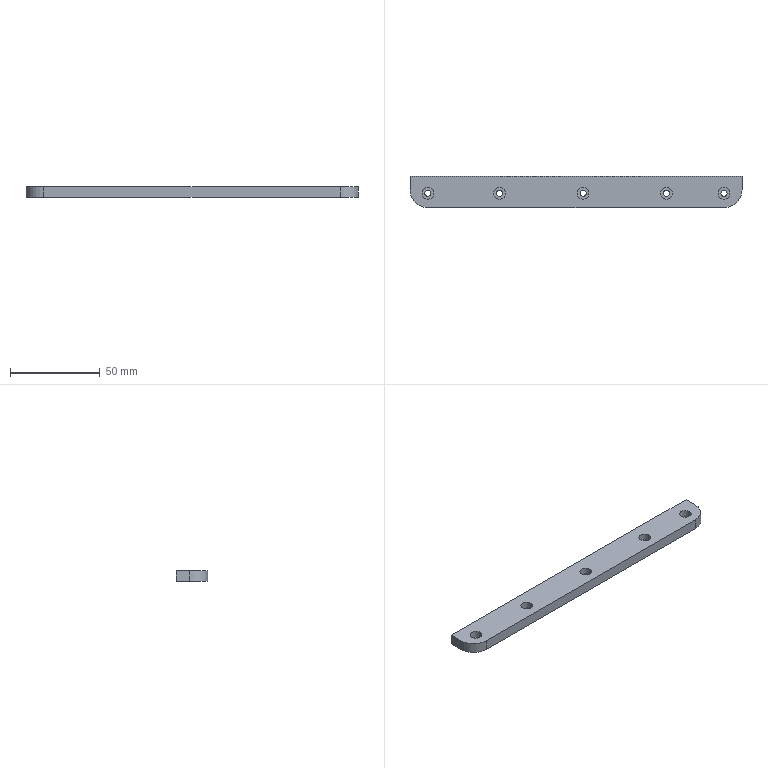Part | STEP file | 229H151433 Default | 1 solid | 33 faces | box 185 x 17.5 x 6 mm | volume 18413 mm3 | cylinder 22 | plane 11 | commonest cylinder face diameters 3.4 x10 6.5 x10 20 x2
STEP:
#1=CARTESIAN_POINT('',(79.209,-0.75,2.));
#2=VERTEX_POINT('',#1);
#3=CARTESIAN_POINT('',(85.709,-0.75,2.));
#4=VERTEX_POINT('',#3);
#5=CARTESIAN_POINT('',(82.459,-0.75,2.));
#6=DIRECTION('',(0.,0.,1.));
#7=DIRECTION('',(1.,0.,0.));
#8=AXIS2_PLACEMENT_3D('',#5,#6,#7);
#9=CIRCLE('',#8,3.25);
#10=EDGE_CURVE('',#2,#4,#9,.T.);
#11=ORIENTED_EDGE('',*,*,#10,.F.);
#12=CARTESIAN_POINT('',(79.209,-0.75,6.));
#13=VERTEX_POINT('',#12);
#14=CARTESIAN_POINT('',(79.209,-0.75,6.));
#15=DIRECTION('',(0.,0.,1.));
#16=VECTOR('',#15,1000.);
#17=LINE('',#14,#16);
#18=EDGE_CURVE('',#2,#13,#17,.T.);
#19=ORIENTED_EDGE('',*,*,#18,.T.);
#20=CARTESIAN_POINT('',(85.709,-0.75,6.));
#21=VERTEX_POINT('',#20);
#22=CARTESIAN_POINT('',(82.459,-0.75,6.));
#23=DIRECTION('',(0.,0.,1.));
#24=DIRECTION('',(1.,0.,0.));
#25=AXIS2_PLACEMENT_3D('',#22,#23,#24);
#26=CIRCLE('',#25,3.25);
#27=EDGE_CURVE('',#13,#21,#26,.T.);
#28=ORIENTED_EDGE('',*,*,#27,.T.);
#29=CARTESIAN_POINT('',(85.709,-0.75,6.));
#30=DIRECTION('',(0.,0.,1.));
#31=VECTOR('',#30,1000.);
#32=LINE('',#29,#31);
#33=EDGE_CURVE('',#4,#21,#32,.T.);
#34=ORIENTED_EDGE('',*,*,#33,.F.);
#35=EDGE_LOOP('',(#11,#19,#28,#34));
#36=FACE_OUTER_BOUND('',#35,.T.);
#37=CARTESIAN_POINT('',(82.459,-0.75,6.));
#38=DIRECTION('',(0.,0.,1.));
#39=DIRECTION('',(1.,0.,0.));
#40=AXIS2_PLACEMENT_3D('',#37,#38,#39);
#41=CYLINDRICAL_SURFACE('',#40,3.25);
#42=ADVANCED_FACE('',(#36),#41,.F.);
#43=CARTESIAN_POINT('',(80.759,-0.75,0.));
#44=VERTEX_POINT('',#43);
#45=CARTESIAN_POINT('',(84.159,-0.75,0.));
#46=VERTEX_POINT('',#45);
#47=CARTESIAN_POINT('',(82.459,-0.75,0.));
#48=DIRECTION('',(0.,0.,1.));
#49=DIRECTION('',(1.,0.,0.));
#50=AXIS2_PLACEMENT_3D('',#47,#48,#49);
#51=CIRCLE('',#50,1.7);
#52=EDGE_CURVE('',#44,#46,#51,.T.);
#53=ORIENTED_EDGE('',*,*,#52,.F.);
#54=CARTESIAN_POINT('',(80.759,-0.75,2.));
#55=VERTEX_POINT('',#54);
#56=CARTESIAN_POINT('',(80.759,-0.75,6.));
#57=DIRECTION('',(0.,0.,1.));
#58=VECTOR('',#57,1000.);
#59=LINE('',#56,#58);
#60=EDGE_CURVE('',#44,#55,#59,.T.);
#61=ORIENTED_EDGE('',*,*,#60,.T.);
#62=CARTESIAN_POINT('',(84.159,-0.75,2.));
#63=VERTEX_POINT('',#62);
#64=CARTESIAN_POINT('',(82.459,-0.75,2.));
#65=DIRECTION('',(0.,0.,1.));
#66=DIRECTION('',(1.,0.,0.));
#67=AXIS2_PLACEMENT_3D('',#64,#65,#66);
#68=CIRCLE('',#67,1.7);
#69=EDGE_CURVE('',#55,#63,#68,.T.);
#70=ORIENTED_EDGE('',*,*,#69,.T.);
#71=CARTESIAN_POINT('',(84.159,-0.75,6.));
#72=DIRECTION('',(0.,0.,1.));
#73=VECTOR('',#72,1000.);
#74=LINE('',#71,#73);
#75=EDGE_CURVE('',#46,#63,#74,.T.);
#76=ORIENTED_EDGE('',*,*,#75,.F.);
#77=EDGE_LOOP('',(#53,#61,#70,#76));
#78=FACE_OUTER_BOUND('',#77,.T.);
#79=CARTESIAN_POINT('',(82.459,-0.75,6.));
#80=DIRECTION('',(0.,0.,1.));
#81=DIRECTION('',(1.,0.,0.));
#82=AXIS2_PLACEMENT_3D('',#79,#80,#81);
#83=CYLINDRICAL_SURFACE('',#82,1.7);
#84=ADVANCED_FACE('',(#78),#83,.F.);
#85=CARTESIAN_POINT('',(47.209,-0.75,2.));
#86=VERTEX_POINT('',#85);
#87=CARTESIAN_POINT('',(53.709,-0.75,2.));
#88=VERTEX_POINT('',#87);
#89=CARTESIAN_POINT('',(50.459,-0.75,2.));
#90=DIRECTION('',(0.,0.,1.));
#91=DIRECTION('',(1.,0.,0.));
#92=AXIS2_PLACEMENT_3D('',#89,#90,#91);
#93=CIRCLE('',#92,3.25);
#94=EDGE_CURVE('',#86,#88,#93,.T.);
#95=ORIENTED_EDGE('',*,*,#94,.F.);
#96=CARTESIAN_POINT('',(47.209,-0.75,6.));
#97=VERTEX_POINT('',#96);
#98=CARTESIAN_POINT('',(47.209,-0.75,6.));
#99=DIRECTION('',(0.,0.,1.));
#100=VECTOR('',#99,1000.);
#101=LINE('',#98,#100);
#102=EDGE_CURVE('',#86,#97,#101,.T.);
#103=ORIENTED_EDGE('',*,*,#102,.T.);
#104=CARTESIAN_POINT('',(53.709,-0.75,6.));
#105=VERTEX_POINT('',#104);
#106=CARTESIAN_POINT('',(50.459,-0.75,6.));
#107=DIRECTION('',(0.,0.,1.));
#108=DIRECTION('',(1.,0.,0.));
#109=AXIS2_PLACEMENT_3D('',#106,#107,#108);
#110=CIRCLE('',#109,3.25);
#111=EDGE_CURVE('',#97,#105,#110,.T.);
#112=ORIENTED_EDGE('',*,*,#111,.T.);
#113=CARTESIAN_POINT('',(53.709,-0.75,6.));
#114=DIRECTION('',(0.,0.,1.));
#115=VECTOR('',#114,1000.);
#116=LINE('',#113,#115);
#117=EDGE_CURVE('',#88,#105,#116,.T.);
#118=ORIENTED_EDGE('',*,*,#117,.F.);
#119=EDGE_LOOP('',(#95,#103,#112,#118));
#120=FACE_OUTER_BOUND('',#119,.T.);
#121=CARTESIAN_POINT('',(50.459,-0.75,6.));
#122=DIRECTION('',(0.,0.,1.));
#123=DIRECTION('',(1.,0.,0.));
#124=AXIS2_PLACEMENT_3D('',#121,#122,#123);
#125=CYLINDRICAL_SURFACE('',#124,3.25);
#126=ADVANCED_FACE('',(#120),#125,.F.);
#127=CARTESIAN_POINT('',(48.759,-0.75,0.));
#128=VERTEX_POINT('',#127);
#129=CARTESIAN_POINT('',(52.159,-0.75,0.));
#130=VERTEX_POINT('',#129);
#131=CARTESIAN_POINT('',(50.459,-0.75,0.));
#132=DIRECTION('',(0.,0.,1.));
#133=DIRECTION('',(1.,0.,0.));
#134=AXIS2_PLACEMENT_3D('',#131,#132,#133);
#135=CIRCLE('',#134,1.7);
#136=EDGE_CURVE('',#128,#130,#135,.T.);
#137=ORIENTED_EDGE('',*,*,#136,.F.);
#138=CARTESIAN_POINT('',(48.759,-0.75,2.));
#139=VERTEX_POINT('',#138);
#140=CARTESIAN_POINT('',(48.759,-0.75,6.));
#141=DIRECTION('',(0.,0.,1.));
#142=VECTOR('',#141,1000.);
#143=LINE('',#140,#142);
#144=EDGE_CURVE('',#128,#139,#143,.T.);
#145=ORIENTED_EDGE('',*,*,#144,.T.);
#146=CARTESIAN_POINT('',(52.159,-0.75,2.));
#147=VERTEX_POINT('',#146);
#148=CARTESIAN_POINT('',(50.459,-0.75,2.));
#149=DIRECTION('',(0.,0.,1.));
#150=DIRECTION('',(1.,0.,0.));
#151=AXIS2_PLACEMENT_3D('',#148,#149,#150);
#152=CIRCLE('',#151,1.7);
#153=EDGE_CURVE('',#139,#147,#152,.T.);
#154=ORIENTED_EDGE('',*,*,#153,.T.);
#155=CARTESIAN_POINT('',(52.159,-0.75,6.));
#156=DIRECTION('',(0.,0.,1.));
#157=VECTOR('',#156,1000.);
#158=LINE('',#155,#157);
#159=EDGE_CURVE('',#130,#147,#158,.T.);
#160=ORIENTED_EDGE('',*,*,#159,.F.);
#161=EDGE_LOOP('',(#137,#145,#154,#160));
#162=FACE_OUTER_BOUND('',#161,.T.);
#163=CARTESIAN_POINT('',(50.459,-0.75,6.));
#164=DIRECTION('',(0.,0.,1.));
#165=DIRECTION('',(1.,0.,0.));
#166=AXIS2_PLACEMENT_3D('',#163,#164,#165);
#167=CYLINDRICAL_SURFACE('',#166,1.7);
#168=ADVANCED_FACE('',(#162),#167,.F.);
#169=CARTESIAN_POINT('',(0.7093,-0.75,2.));
#170=VERTEX_POINT('',#169);
#171=CARTESIAN_POINT('',(7.209,-0.75,2.));
#172=VERTEX_POINT('',#171);
#173=CARTESIAN_POINT('',(3.959,-0.75,2.));
#174=DIRECTION('',(0.,0.,1.));
#175=DIRECTION('',(1.,0.,0.));
#176=AXIS2_PLACEMENT_3D('',#173,#174,#175);
#177=CIRCLE('',#176,3.25);
#178=EDGE_CURVE('',#170,#172,#177,.T.);
#179=ORIENTED_EDGE('',*,*,#178,.F.);
#180=CARTESIAN_POINT('',(0.7093,-0.75,6.));
#181=VERTEX_POINT('',#180);
#182=CARTESIAN_POINT('',(0.7093,-0.75,6.));
#183=DIRECTION('',(0.,0.,1.));
#184=VECTOR('',#183,1000.);
#185=LINE('',#182,#184);
#186=EDGE_CURVE('',#170,#181,#185,.T.);
#187=ORIENTED_EDGE('',*,*,#186,.T.);
#188=CARTESIAN_POINT('',(7.209,-0.75,6.));
#189=VERTEX_POINT('',#188);
#190=CARTESIAN_POINT('',(3.959,-0.75,6.));
#191=DIRECTION('',(0.,0.,1.));
#192=DIRECTION('',(1.,0.,0.));
#193=AXIS2_PLACEMENT_3D('',#190,#191,#192);
#194=CIRCLE('',#193,3.25);
#195=EDGE_CURVE('',#181,#189,#194,.T.);
#196=ORIENTED_EDGE('',*,*,#195,.T.);
#197=CARTESIAN_POINT('',(7.209,-0.75,6.));
#198=DIRECTION('',(0.,0.,1.));
#199=VECTOR('',#198,1000.);
#200=LINE('',#197,#199);
#201=EDGE_CURVE('',#172,#189,#200,.T.);
#202=ORIENTED_EDGE('',*,*,#201,.F.);
#203=EDGE_LOOP('',(#179,#187,#196,#202));
#204=FACE_OUTER_BOUND('',#203,.T.);
#205=CARTESIAN_POINT('',(3.959,-0.75,6.));
#206=DIRECTION('',(0.,0.,1.));
#207=DIRECTION('',(1.,0.,0.));
#208=AXIS2_PLACEMENT_3D('',#205,#206,#207);
#209=CYLINDRICAL_SURFACE('',#208,3.25);
#210=ADVANCED_FACE('',(#204),#209,.F.);
#211=CARTESIAN_POINT('',(2.259,-0.75,0.));
#212=VERTEX_POINT('',#211);
#213=CARTESIAN_POINT('',(5.659,-0.75,0.));
#214=VERTEX_POINT('',#213);
#215=CARTESIAN_POINT('',(3.959,-0.75,0.));
#216=DIRECTION('',(0.,0.,1.));
#217=DIRECTION('',(1.,0.,0.));
#218=AXIS2_PLACEMENT_3D('',#215,#216,#217);
#219=CIRCLE('',#218,1.7);
#220=EDGE_CURVE('',#212,#214,#219,.T.);
#221=ORIENTED_EDGE('',*,*,#220,.F.);
#222=CARTESIAN_POINT('',(2.259,-0.75,2.));
#223=VERTEX_POINT('',#222);
#224=CARTESIAN_POINT('',(2.259,-0.75,6.));
#225=DIRECTION('',(0.,0.,1.));
#226=VECTOR('',#225,1000.);
#227=LINE('',#224,#226);
#228=EDGE_CURVE('',#212,#223,#227,.T.);
#229=ORIENTED_EDGE('',*,*,#228,.T.);
#230=CARTESIAN_POINT('',(5.659,-0.75,2.));
#231=VERTEX_POINT('',#230);
#232=CARTESIAN_POINT('',(3.959,-0.75,2.));
#233=DIRECTION('',(0.,0.,1.));
#234=DIRECTION('',(1.,0.,0.));
#235=AXIS2_PLACEMENT_3D('',#232,#233,#234);
#236=CIRCLE('',#235,1.7);
#237=EDGE_CURVE('',#223,#231,#236,.T.);
#238=ORIENTED_EDGE('',*,*,#237,.T.);
#239=CARTESIAN_POINT('',(5.659,-0.75,6.));
#240=DIRECTION('',(0.,0.,1.));
#241=VECTOR('',#240,1000.);
#242=LINE('',#239,#241);
#243=EDGE_CURVE('',#214,#231,#242,.T.);
#244=ORIENTED_EDGE('',*,*,#243,.F.);
#245=EDGE_LOOP('',(#221,#229,#238,#244));
#246=FACE_OUTER_BOUND('',#245,.T.);
#247=CARTESIAN_POINT('',(3.959,-0.75,6.));
#248=DIRECTION('',(0.,0.,1.));
#249=DIRECTION('',(1.,0.,0.));
#250=AXIS2_PLACEMENT_3D('',#247,#248,#249);
#251=CYLINDRICAL_SURFACE('',#250,1.7);
#252=ADVANCED_FACE('',(#246),#251,.F.);
#253=CARTESIAN_POINT('',(-45.791,-0.75,2.));
#254=VERTEX_POINT('',#253);
#255=CARTESIAN_POINT('',(-39.291,-0.75,2.));
#256=VERTEX_POINT('',#255);
#257=CARTESIAN_POINT('',(-42.541,-0.75,2.));
#258=DIRECTION('',(0.,0.,1.));
#259=DIRECTION('',(1.,0.,0.));
#260=AXIS2_PLACEMENT_3D('',#257,#258,#259);
#261=CIRCLE('',#260,3.25);
#262=EDGE_CURVE('',#254,#256,#261,.T.);
#263=ORIENTED_EDGE('',*,*,#262,.F.);
#264=CARTESIAN_POINT('',(-45.791,-0.75,6.));
#265=VERTEX_POINT('',#264);
#266=CARTESIAN_POINT('',(-45.791,-0.75,6.));
#267=DIRECTION('',(0.,0.,1.));
#268=VECTOR('',#267,1000.);
#269=LINE('',#266,#268);
#270=EDGE_CURVE('',#254,#265,#269,.T.);
#271=ORIENTED_EDGE('',*,*,#270,.T.);
#272=CARTESIAN_POINT('',(-39.291,-0.75,6.));
#273=VERTEX_POINT('',#272);
#274=CARTESIAN_POINT('',(-42.541,-0.75,6.));
#275=DIRECTION('',(0.,0.,1.));
#276=DIRECTION('',(1.,0.,0.));
#277=AXIS2_PLACEMENT_3D('',#274,#275,#276);
#278=CIRCLE('',#277,3.25);
#279=EDGE_CURVE('',#265,#273,#278,.T.);
#280=ORIENTED_EDGE('',*,*,#279,.T.);
#281=CARTESIAN_POINT('',(-39.291,-0.75,6.));
#282=DIRECTION('',(0.,0.,1.));
#283=VECTOR('',#282,1000.);
#284=LINE('',#281,#283);
#285=EDGE_CURVE('',#256,#273,#284,.T.);
#286=ORIENTED_EDGE('',*,*,#285,.F.);
#287=EDGE_LOOP('',(#263,#271,#280,#286));
#288=FACE_OUTER_BOUND('',#287,.T.);
#289=CARTESIAN_POINT('',(-42.541,-0.75,6.));
#290=DIRECTION('',(0.,0.,1.));
#291=DIRECTION('',(1.,0.,0.));
#292=AXIS2_PLACEMENT_3D('',#289,#290,#291);
#293=CYLINDRICAL_SURFACE('',#292,3.25);
#294=ADVANCED_FACE('',(#288),#293,.F.);
#295=CARTESIAN_POINT('',(-44.241,-0.75,0.));
#296=VERTEX_POINT('',#295);
#297=CARTESIAN_POINT('',(-40.841,-0.75,0.));
#298=VERTEX_POINT('',#297);
#299=CARTESIAN_POINT('',(-42.541,-0.75,0.));
#300=DIRECTION('',(0.,0.,1.));
#301=DIRECTION('',(1.,0.,0.));
#302=AXIS2_PLACEMENT_3D('',#299,#300,#301);
#303=CIRCLE('',#302,1.7);
#304=EDGE_CURVE('',#296,#298,#303,.T.);
#305=ORIENTED_EDGE('',*,*,#304,.F.);
#306=CARTESIAN_POINT('',(-44.241,-0.75,2.));
#307=VERTEX_POINT('',#306);
#308=CARTESIAN_POINT('',(-44.241,-0.75,6.));
#309=DIRECTION('',(0.,0.,1.));
#310=VECTOR('',#309,1000.);
#311=LINE('',#308,#310);
#312=EDGE_CURVE('',#296,#307,#311,.T.);
#313=ORIENTED_EDGE('',*,*,#312,.T.);
#314=CARTESIAN_POINT('',(-40.841,-0.75,2.));
#315=VERTEX_POINT('',#314);
#316=CARTESIAN_POINT('',(-42.541,-0.75,2.));
#317=DIRECTION('',(0.,0.,1.));
#318=DIRECTION('',(1.,0.,0.));
#319=AXIS2_PLACEMENT_3D('',#316,#317,#318);
#320=CIRCLE('',#319,1.7);
#321=EDGE_CURVE('',#307,#315,#320,.T.);
#322=ORIENTED_EDGE('',*,*,#321,.T.);
#323=CARTESIAN_POINT('',(-40.841,-0.75,6.));
#324=DIRECTION('',(0.,0.,1.));
#325=VECTOR('',#324,1000.);
#326=LINE('',#323,#325);
#327=EDGE_CURVE('',#298,#315,#326,.T.);
#328=ORIENTED_EDGE('',*,*,#327,.F.);
#329=EDGE_LOOP('',(#305,#313,#322,#328));
#330=FACE_OUTER_BOUND('',#329,.T.);
#331=CARTESIAN_POINT('',(-42.541,-0.75,6.));
#332=DIRECTION('',(0.,0.,1.));
#333=DIRECTION('',(1.,0.,0.));
#334=AXIS2_PLACEMENT_3D('',#331,#332,#333);
#335=CYLINDRICAL_SURFACE('',#334,1.7);
#336=ADVANCED_FACE('',(#330),#335,.F.);
#337=CARTESIAN_POINT('',(-85.791,-0.75,2.));
#338=VERTEX_POINT('',#337);
#339=CARTESIAN_POINT('',(-79.291,-0.75,2.));
#340=VERTEX_POINT('',#339);
#341=CARTESIAN_POINT('',(-82.541,-0.75,2.));
#342=DIRECTION('',(0.,0.,1.));
#343=DIRECTION('',(1.,0.,0.));
#344=AXIS2_PLACEMENT_3D('',#341,#342,#343);
#345=CIRCLE('',#344,3.25);
#346=EDGE_CURVE('',#338,#340,#345,.T.);
#347=ORIENTED_EDGE('',*,*,#346,.F.);
#348=CARTESIAN_POINT('',(-85.791,-0.75,6.));
#349=VERTEX_POINT('',#348);
#350=CARTESIAN_POINT('',(-85.791,-0.75,6.));
#351=DIRECTION('',(0.,0.,1.));
#352=VECTOR('',#351,1000.);
#353=LINE('',#350,#352);
#354=EDGE_CURVE('',#338,#349,#353,.T.);
#355=ORIENTED_EDGE('',*,*,#354,.T.);
#356=CARTESIAN_POINT('',(-79.291,-0.75,6.));
#357=VERTEX_POINT('',#356);
#358=CARTESIAN_POINT('',(-82.541,-0.75,6.));
#359=DIRECTION('',(0.,0.,1.));
#360=DIRECTION('',(1.,0.,0.));
#361=AXIS2_PLACEMENT_3D('',#358,#359,#360);
#362=CIRCLE('',#361,3.25);
#363=EDGE_CURVE('',#349,#357,#362,.T.);
#364=ORIENTED_EDGE('',*,*,#363,.T.);
#365=CARTESIAN_POINT('',(-79.291,-0.75,6.));
#366=DIRECTION('',(0.,0.,1.));
#367=VECTOR('',#366,1000.);
#368=LINE('',#365,#367);
#369=EDGE_CURVE('',#340,#357,#368,.T.);
#370=ORIENTED_EDGE('',*,*,#369,.F.);
#371=EDGE_LOOP('',(#347,#355,#364,#370));
#372=FACE_OUTER_BOUND('',#371,.T.);
#373=CARTESIAN_POINT('',(-82.541,-0.75,6.));
#374=DIRECTION('',(0.,0.,1.));
#375=DIRECTION('',(1.,0.,0.));
#376=AXIS2_PLACEMENT_3D('',#373,#374,#375);
#377=CYLINDRICAL_SURFACE('',#376,3.25);
#378=ADVANCED_FACE('',(#372),#377,.F.);
#379=CARTESIAN_POINT('',(-84.241,-0.75,0.));
#380=VERTEX_POINT('',#379);
#381=CARTESIAN_POINT('',(-80.841,-0.75,0.));
#382=VERTEX_POINT('',#381);
#383=CARTESIAN_POINT('',(-82.541,-0.75,0.));
#384=DIRECTION('',(0.,0.,1.));
#385=DIRECTION('',(1.,0.,0.));
#386=AXIS2_PLACEMENT_3D('',#383,#384,#385);
#387=CIRCLE('',#386,1.7);
#388=EDGE_CURVE('',#380,#382,#387,.T.);
#389=ORIENTED_EDGE('',*,*,#388,.F.);
#390=CARTESIAN_POINT('',(-84.241,-0.75,2.));
#391=VERTEX_POINT('',#390);
#392=CARTESIAN_POINT('',(-84.241,-0.75,6.));
#393=DIRECTION('',(0.,0.,1.));
#394=VECTOR('',#393,1000.);
#395=LINE('',#392,#394);
#396=EDGE_CURVE('',#380,#391,#395,.T.);
#397=ORIENTED_EDGE('',*,*,#396,.T.);
#398=CARTESIAN_POINT('',(-80.841,-0.75,2.));
#399=VERTEX_POINT('',#398);
#400=CARTESIAN_POINT('',(-82.541,-0.75,2.));
#401=DIRECTION('',(0.,0.,1.));
#402=DIRECTION('',(1.,0.,0.));
#403=AXIS2_PLACEMENT_3D('',#400,#401,#402);
#404=CIRCLE('',#403,1.7);
#405=EDGE_CURVE('',#391,#399,#404,.T.);
#406=ORIENTED_EDGE('',*,*,#405,.T.);
#407=CARTESIAN_POINT('',(-80.841,-0.75,6.));
#408=DIRECTION('',(0.,0.,1.));
#409=VECTOR('',#408,1000.);
#410=LINE('',#407,#409);
#411=EDGE_CURVE('',#382,#399,#410,.T.);
#412=ORIENTED_EDGE('',*,*,#411,.F.);
#413=EDGE_LOOP('',(#389,#397,#406,#412));
#414=FACE_OUTER_BOUND('',#413,.T.);
#415=CARTESIAN_POINT('',(-82.541,-0.75,6.));
#416=DIRECTION('',(0.,0.,1.));
#417=DIRECTION('',(1.,0.,0.));
#418=AXIS2_PLACEMENT_3D('',#415,#416,#417);
#419=CYLINDRICAL_SURFACE('',#418,1.7);
#420=ADVANCED_FACE('',(#414),#419,.F.);
#421=CARTESIAN_POINT('',(92.5,1.25,6.));
#422=VERTEX_POINT('',#421);
#423=CARTESIAN_POINT('',(92.5,8.75,6.));
#424=VERTEX_POINT('',#423);
#425=CARTESIAN_POINT('',(92.5,8.75,6.));
#426=DIRECTION('',(0.,1.,0.));
#427=VECTOR('',#426,1000.);
#428=LINE('',#425,#427);
#429=EDGE_CURVE('',#422,#424,#428,.T.);
#430=ORIENTED_EDGE('',*,*,#429,.F.);
#431=CARTESIAN_POINT('',(92.5,1.25,0.));
#432=VERTEX_POINT('',#431);
#433=CARTESIAN_POINT('',(92.5,1.25,6.));
#434=DIRECTION('',(0.,0.,-1.));
#435=VECTOR('',#434,1000.);
#436=LINE('',#433,#435);
#437=EDGE_CURVE('',#422,#432,#436,.T.);
#438=ORIENTED_EDGE('',*,*,#437,.T.);
#439=CARTESIAN_POINT('',(92.5,8.75,0.));
#440=VERTEX_POINT('',#439);
#441=CARTESIAN_POINT('',(92.5,8.75,0.));
#442=DIRECTION('',(0.,1.,0.));
#443=VECTOR('',#442,1000.);
#444=LINE('',#441,#443);
#445=EDGE_CURVE('',#432,#440,#444,.T.);
#446=ORIENTED_EDGE('',*,*,#445,.T.);
#447=CARTESIAN_POINT('',(92.5,8.75,6.));
#448=DIRECTION('',(0.,0.,-1.));
#449=VECTOR('',#448,1000.);
#450=LINE('',#447,#449);
#451=EDGE_CURVE('',#424,#440,#450,.T.);
#452=ORIENTED_EDGE('',*,*,#451,.F.);
#453=EDGE_LOOP('',(#430,#438,#446,#452));
#454=FACE_OUTER_BOUND('',#453,.T.);
#455=CARTESIAN_POINT('',(92.5,8.75,6.));
#456=DIRECTION('',(-1.,0.,0.));
#457=DIRECTION('',(0.,0.,1.));
#458=AXIS2_PLACEMENT_3D('',#455,#456,#457);
#459=PLANE('',#458);
#460=ADVANCED_FACE('',(#454),#459,.F.);
#461=CARTESIAN_POINT('',(-92.5,8.75,0.));
#462=VERTEX_POINT('',#461);
#463=CARTESIAN_POINT('',(-92.5,8.75,0.));
#464=DIRECTION('',(-1.,0.,0.));
#465=VECTOR('',#464,1000.);
#466=LINE('',#463,#465);
#467=EDGE_CURVE('',#440,#462,#466,.T.);
#468=ORIENTED_EDGE('',*,*,#467,.T.);
#469=CARTESIAN_POINT('',(-92.5,8.75,6.));
#470=VERTEX_POINT('',#469);
#471=CARTESIAN_POINT('',(-92.5,8.75,6.));
#472=DIRECTION('',(0.,0.,-1.));
#473=VECTOR('',#472,1000.);
#474=LINE('',#471,#473);
#475=EDGE_CURVE('',#470,#462,#474,.T.);
#476=ORIENTED_EDGE('',*,*,#475,.F.);
#477=CARTESIAN_POINT('',(-92.5,8.75,6.));
#478=DIRECTION('',(-1.,0.,0.));
#479=VECTOR('',#478,1000.);
#480=LINE('',#477,#479);
#481=EDGE_CURVE('',#424,#470,#480,.T.);
#482=ORIENTED_EDGE('',*,*,#481,.F.);
#483=ORIENTED_EDGE('',*,*,#451,.T.);
#484=EDGE_LOOP('',(#468,#476,#482,#483));
#485=FACE_OUTER_BOUND('',#484,.T.);
#486=CARTESIAN_POINT('',(-92.5,8.75,6.));
#487=DIRECTION('',(0.,-1.,0.));
#488=DIRECTION('',(0.,0.,-1.));
#489=AXIS2_PLACEMENT_3D('',#486,#487,#488);
#490=PLANE('',#489);
#491=ADVANCED_FACE('',(#485),#490,.F.);
#492=CARTESIAN_POINT('',(-92.5,1.25,0.));
#493=VERTEX_POINT('',#492);
#494=CARTESIAN_POINT('',(-92.5,8.75,0.));
#495=DIRECTION('',(0.,-1.,0.));
#496=VECTOR('',#495,1000.);
#497=LINE('',#494,#496);
#498=EDGE_CURVE('',#462,#493,#497,.T.);
#499=ORIENTED_EDGE('',*,*,#498,.T.);
#500=CARTESIAN_POINT('',(-92.5,1.25,6.));
#501=VERTEX_POINT('',#500);
#502=CARTESIAN_POINT('',(-92.5,1.25,6.));
#503=DIRECTION('',(0.,0.,1.));
#504=VECTOR('',#503,1000.);
#505=LINE('',#502,#504);
#506=EDGE_CURVE('',#493,#501,#505,.T.);
#507=ORIENTED_EDGE('',*,*,#506,.T.);
#508=CARTESIAN_POINT('',(-92.5,8.75,6.));
#509=DIRECTION('',(0.,-1.,0.));
#510=VECTOR('',#509,1000.);
#511=LINE('',#508,#510);
#512=EDGE_CURVE('',#470,#501,#511,.T.);
#513=ORIENTED_EDGE('',*,*,#512,.F.);
#514=ORIENTED_EDGE('',*,*,#475,.T.);
#515=EDGE_LOOP('',(#499,#507,#513,#514));
#516=FACE_OUTER_BOUND('',#515,.T.);
#517=CARTESIAN_POINT('',(-92.5,8.75,6.));
#518=DIRECTION('',(1.,0.,0.));
#519=DIRECTION('',(0.,0.,-1.));
#520=AXIS2_PLACEMENT_3D('',#517,#518,#519);
#521=PLANE('',#520);
#522=ADVANCED_FACE('',(#516),#521,.F.);
#523=CARTESIAN_POINT('',(-82.5,-8.75,0.));
#524=VERTEX_POINT('',#523);
#525=CARTESIAN_POINT('',(82.5,-8.75,0.));
#526=VERTEX_POINT('',#525);
#527=CARTESIAN_POINT('',(-92.5,-8.75,0.));
#528=DIRECTION('',(1.,0.,0.));
#529=VECTOR('',#528,1000.);
#530=LINE('',#527,#529);
#531=EDGE_CURVE('',#524,#526,#530,.T.);
#532=ORIENTED_EDGE('',*,*,#531,.T.);
#533=CARTESIAN_POINT('',(82.5,-8.75,6.));
#534=VERTEX_POINT('',#533);
#535=CARTESIAN_POINT('',(82.5,-8.75,6.));
#536=DIRECTION('',(0.,0.,1.));
#537=VECTOR('',#536,1000.);
#538=LINE('',#535,#537);
#539=EDGE_CURVE('',#526,#534,#538,.T.);
#540=ORIENTED_EDGE('',*,*,#539,.T.);
#541=CARTESIAN_POINT('',(-82.5,-8.75,6.));
#542=VERTEX_POINT('',#541);
#543=CARTESIAN_POINT('',(-92.5,-8.75,6.));
#544=DIRECTION('',(1.,0.,0.));
#545=VECTOR('',#544,1000.);
#546=LINE('',#543,#545);
#547=EDGE_CURVE('',#542,#534,#546,.T.);
#548=ORIENTED_EDGE('',*,*,#547,.F.);
#549=CARTESIAN_POINT('',(-82.5,-8.75,6.));
#550=DIRECTION('',(0.,0.,-1.));
#551=VECTOR('',#550,1000.);
#552=LINE('',#549,#551);
#553=EDGE_CURVE('',#542,#524,#552,.T.);
#554=ORIENTED_EDGE('',*,*,#553,.T.);
#555=EDGE_LOOP('',(#532,#540,#548,#554));
#556=FACE_OUTER_BOUND('',#555,.T.);
#557=CARTESIAN_POINT('',(-92.5,-8.75,6.));
#558=DIRECTION('',(0.,1.,0.));
#559=DIRECTION('',(0.,0.,1.));
#560=AXIS2_PLACEMENT_3D('',#557,#558,#559);
#561=PLANE('',#560);
#562=ADVANCED_FACE('',(#556),#561,.F.);
#563=CARTESIAN_POINT('',(82.459,-0.75,6.));
#564=DIRECTION('',(0.,0.,1.));
#565=DIRECTION('',(1.,0.,0.));
#566=AXIS2_PLACEMENT_3D('',#563,#564,#565);
#567=CIRCLE('',#566,3.25);
#568=EDGE_CURVE('',#21,#13,#567,.T.);
#569=ORIENTED_EDGE('',*,*,#568,.F.);
#570=ORIENTED_EDGE('',*,*,#27,.F.);
#571=EDGE_LOOP('',(#569,#570));
#572=FACE_BOUND('',#571,.T.);
#573=CARTESIAN_POINT('',(50.459,-0.75,6.));
#574=DIRECTION('',(0.,0.,1.));
#575=DIRECTION('',(1.,0.,0.));
#576=AXIS2_PLACEMENT_3D('',#573,#574,#575);
#577=CIRCLE('',#576,3.25);
#578=EDGE_CURVE('',#105,#97,#577,.T.);
#579=ORIENTED_EDGE('',*,*,#578,.F.);
#580=ORIENTED_EDGE('',*,*,#111,.F.);
#581=EDGE_LOOP('',(#579,#580));
#582=FACE_BOUND('',#581,.T.);
#583=CARTESIAN_POINT('',(3.959,-0.75,6.));
#584=DIRECTION('',(0.,0.,1.));
#585=DIRECTION('',(1.,0.,0.));
#586=AXIS2_PLACEMENT_3D('',#583,#584,#585);
#587=CIRCLE('',#586,3.25);
#588=EDGE_CURVE('',#189,#181,#587,.T.);
#589=ORIENTED_EDGE('',*,*,#588,.F.);
#590=ORIENTED_EDGE('',*,*,#195,.F.);
#591=EDGE_LOOP('',(#589,#590));
#592=FACE_BOUND('',#591,.T.);
#593=CARTESIAN_POINT('',(-42.541,-0.75,6.));
#594=DIRECTION('',(0.,0.,1.));
#595=DIRECTION('',(1.,0.,0.));
#596=AXIS2_PLACEMENT_3D('',#593,#594,#595);
#597=CIRCLE('',#596,3.25);
#598=EDGE_CURVE('',#273,#265,#597,.T.);
#599=ORIENTED_EDGE('',*,*,#598,.F.);
#600=ORIENTED_EDGE('',*,*,#279,.F.);
#601=EDGE_LOOP('',(#599,#600));
#602=FACE_BOUND('',#601,.T.);
#603=CARTESIAN_POINT('',(-82.541,-0.75,6.));
#604=DIRECTION('',(0.,0.,1.));
#605=DIRECTION('',(1.,0.,0.));
#606=AXIS2_PLACEMENT_3D('',#603,#604,#605);
#607=CIRCLE('',#606,3.25);
#608=EDGE_CURVE('',#357,#349,#607,.T.);
#609=ORIENTED_EDGE('',*,*,#608,.F.);
#610=ORIENTED_EDGE('',*,*,#363,.F.);
#611=EDGE_LOOP('',(#609,#610));
#612=FACE_BOUND('',#611,.T.);
#613=ORIENTED_EDGE('',*,*,#547,.T.);
#614=CARTESIAN_POINT('',(82.5,1.25,6.));
#615=DIRECTION('',(0.,0.,1.));
#616=DIRECTION('',(1.,0.,0.));
#617=AXIS2_PLACEMENT_3D('',#614,#615,#616);
#618=CIRCLE('',#617,10.);
#619=EDGE_CURVE('',#534,#422,#618,.T.);
#620=ORIENTED_EDGE('',*,*,#619,.T.);
#621=ORIENTED_EDGE('',*,*,#429,.T.);
#622=ORIENTED_EDGE('',*,*,#481,.T.);
#623=ORIENTED_EDGE('',*,*,#512,.T.);
#624=CARTESIAN_POINT('',(-82.5,1.25,6.));
#625=DIRECTION('',(0.,0.,1.));
#626=DIRECTION('',(1.,0.,0.));
#627=AXIS2_PLACEMENT_3D('',#624,#625,#626);
#628=CIRCLE('',#627,10.);
#629=EDGE_CURVE('',#501,#542,#628,.T.);
#630=ORIENTED_EDGE('',*,*,#629,.T.);
#631=EDGE_LOOP('',(#613,#620,#621,#622,#623,#630));
#632=FACE_OUTER_BOUND('',#631,.T.);
#633=CARTESIAN_POINT('',(0.,0.,6.));
#634=DIRECTION('',(0.,0.,1.));
#635=DIRECTION('',(1.,0.,0.));
#636=AXIS2_PLACEMENT_3D('',#633,#634,#635);
#637=PLANE('',#636);
#638=ADVANCED_FACE('',(#572,#582,#592,#602,#612,#632),#637,.T.);
#639=CARTESIAN_POINT('',(82.459,-0.75,0.));
#640=DIRECTION('',(0.,0.,1.));
#641=DIRECTION('',(1.,0.,0.));
#642=AXIS2_PLACEMENT_3D('',#639,#640,#641);
#643=CIRCLE('',#642,1.7);
#644=EDGE_CURVE('',#46,#44,#643,.T.);
#645=ORIENTED_EDGE('',*,*,#644,.T.);
#646=ORIENTED_EDGE('',*,*,#52,.T.);
#647=EDGE_LOOP('',(#645,#646));
#648=FACE_BOUND('',#647,.T.);
#649=CARTESIAN_POINT('',(50.459,-0.75,0.));
#650=DIRECTION('',(0.,0.,1.));
#651=DIRECTION('',(1.,0.,0.));
#652=AXIS2_PLACEMENT_3D('',#649,#650,#651);
#653=CIRCLE('',#652,1.7);
#654=EDGE_CURVE('',#130,#128,#653,.T.);
#655=ORIENTED_EDGE('',*,*,#654,.T.);
#656=ORIENTED_EDGE('',*,*,#136,.T.);
#657=EDGE_LOOP('',(#655,#656));
#658=FACE_BOUND('',#657,.T.);
#659=CARTESIAN_POINT('',(3.959,-0.75,0.));
#660=DIRECTION('',(0.,0.,1.));
#661=DIRECTION('',(1.,0.,0.));
#662=AXIS2_PLACEMENT_3D('',#659,#660,#661);
#663=CIRCLE('',#662,1.7);
#664=EDGE_CURVE('',#214,#212,#663,.T.);
#665=ORIENTED_EDGE('',*,*,#664,.T.);
#666=ORIENTED_EDGE('',*,*,#220,.T.);
#667=EDGE_LOOP('',(#665,#666));
#668=FACE_BOUND('',#667,.T.);
#669=CARTESIAN_POINT('',(-42.541,-0.75,0.));
#670=DIRECTION('',(0.,0.,1.));
#671=DIRECTION('',(1.,0.,0.));
#672=AXIS2_PLACEMENT_3D('',#669,#670,#671);
#673=CIRCLE('',#672,1.7);
#674=EDGE_CURVE('',#298,#296,#673,.T.);
#675=ORIENTED_EDGE('',*,*,#674,.T.);
#676=ORIENTED_EDGE('',*,*,#304,.T.);
#677=EDGE_LOOP('',(#675,#676));
#678=FACE_BOUND('',#677,.T.);
#679=CARTESIAN_POINT('',(-82.541,-0.75,0.));
#680=DIRECTION('',(0.,0.,1.));
#681=DIRECTION('',(1.,0.,0.));
#682=AXIS2_PLACEMENT_3D('',#679,#680,#681);
#683=CIRCLE('',#682,1.7);
#684=EDGE_CURVE('',#382,#380,#683,.T.);
#685=ORIENTED_EDGE('',*,*,#684,.T.);
#686=ORIENTED_EDGE('',*,*,#388,.T.);
#687=EDGE_LOOP('',(#685,#686));
#688=FACE_BOUND('',#687,.T.);
#689=ORIENTED_EDGE('',*,*,#445,.F.);
#690=CARTESIAN_POINT('',(82.5,1.25,0.));
#691=DIRECTION('',(0.,0.,-1.));
#692=DIRECTION('',(1.,0.,0.));
#693=AXIS2_PLACEMENT_3D('',#690,#691,#692);
#694=CIRCLE('',#693,10.);
#695=EDGE_CURVE('',#432,#526,#694,.T.);
#696=ORIENTED_EDGE('',*,*,#695,.T.);
#697=ORIENTED_EDGE('',*,*,#531,.F.);
#698=CARTESIAN_POINT('',(-82.5,1.25,0.));
#699=DIRECTION('',(0.,0.,-1.));
#700=DIRECTION('',(1.,0.,0.));
#701=AXIS2_PLACEMENT_3D('',#698,#699,#700);
#702=CIRCLE('',#701,10.);
#703=EDGE_CURVE('',#524,#493,#702,.T.);
#704=ORIENTED_EDGE('',*,*,#703,.T.);
#705=ORIENTED_EDGE('',*,*,#498,.F.);
#706=ORIENTED_EDGE('',*,*,#467,.F.);
#707=EDGE_LOOP('',(#689,#696,#697,#704,#705,#706));
#708=FACE_OUTER_BOUND('',#707,.T.);
#709=CARTESIAN_POINT('',(0.,0.,0.));
#710=DIRECTION('',(0.,0.,1.));
#711=DIRECTION('',(1.,0.,0.));
#712=AXIS2_PLACEMENT_3D('',#709,#710,#711);
#713=PLANE('',#712);
#714=ADVANCED_FACE('',(#648,#658,#668,#678,#688,#708),#713,.F.);
#715=ORIENTED_EDGE('',*,*,#619,.F.);
#716=ORIENTED_EDGE('',*,*,#539,.F.);
#717=ORIENTED_EDGE('',*,*,#695,.F.);
#718=ORIENTED_EDGE('',*,*,#437,.F.);
#719=EDGE_LOOP('',(#715,#716,#717,#718));
#720=FACE_OUTER_BOUND('',#719,.T.);
#721=CARTESIAN_POINT('',(82.5,1.25,6.));
#722=DIRECTION('',(0.,0.,-1.));
#723=DIRECTION('',(-1.,0.,0.));
#724=AXIS2_PLACEMENT_3D('',#721,#722,#723);
#725=CYLINDRICAL_SURFACE('',#724,10.);
#726=ADVANCED_FACE('',(#720),#725,.T.);
#727=ORIENTED_EDGE('',*,*,#629,.F.);
#728=ORIENTED_EDGE('',*,*,#506,.F.);
#729=ORIENTED_EDGE('',*,*,#703,.F.);
#730=ORIENTED_EDGE('',*,*,#553,.F.);
#731=EDGE_LOOP('',(#727,#728,#729,#730));
#732=FACE_OUTER_BOUND('',#731,.T.);
#733=CARTESIAN_POINT('',(-82.5,1.25,6.));
#734=DIRECTION('',(0.,0.,-1.));
#735=DIRECTION('',(-1.,0.,0.));
#736=AXIS2_PLACEMENT_3D('',#733,#734,#735);
#737=CYLINDRICAL_SURFACE('',#736,10.);
#738=ADVANCED_FACE('',(#732),#737,.T.);
#739=ORIENTED_EDGE('',*,*,#396,.F.);
#740=ORIENTED_EDGE('',*,*,#684,.F.);
#741=ORIENTED_EDGE('',*,*,#411,.T.);
#742=CARTESIAN_POINT('',(-82.541,-0.75,2.));
#743=DIRECTION('',(0.,0.,1.));
#744=DIRECTION('',(1.,0.,0.));
#745=AXIS2_PLACEMENT_3D('',#742,#743,#744);
#746=CIRCLE('',#745,1.7);
#747=EDGE_CURVE('',#399,#391,#746,.T.);
#748=ORIENTED_EDGE('',*,*,#747,.T.);
#749=EDGE_LOOP('',(#739,#740,#741,#748));
#750=FACE_OUTER_BOUND('',#749,.T.);
#751=CARTESIAN_POINT('',(-82.541,-0.75,6.));
#752=DIRECTION('',(0.,0.,1.));
#753=DIRECTION('',(1.,0.,0.));
#754=AXIS2_PLACEMENT_3D('',#751,#752,#753);
#755=CYLINDRICAL_SURFACE('',#754,1.7);
#756=ADVANCED_FACE('',(#750),#755,.F.);
#757=ORIENTED_EDGE('',*,*,#747,.F.);
#758=ORIENTED_EDGE('',*,*,#405,.F.);
#759=EDGE_LOOP('',(#757,#758));
#760=FACE_BOUND('',#759,.T.);
#761=CARTESIAN_POINT('',(-82.541,-0.75,2.));
#762=DIRECTION('',(0.,0.,1.));
#763=DIRECTION('',(1.,0.,0.));
#764=AXIS2_PLACEMENT_3D('',#761,#762,#763);
#765=CIRCLE('',#764,3.25);
#766=EDGE_CURVE('',#340,#338,#765,.T.);
#767=ORIENTED_EDGE('',*,*,#766,.T.);
#768=ORIENTED_EDGE('',*,*,#346,.T.);
#769=EDGE_LOOP('',(#767,#768));
#770=FACE_OUTER_BOUND('',#769,.T.);
#771=CARTESIAN_POINT('',(-80.841,-0.75,2.));
#772=DIRECTION('',(0.,0.,-1.));
#773=DIRECTION('',(-1.,0.,0.));
#774=AXIS2_PLACEMENT_3D('',#771,#772,#773);
#775=PLANE('',#774);
#776=ADVANCED_FACE('',(#760,#770),#775,.F.);
#777=ORIENTED_EDGE('',*,*,#354,.F.);
#778=ORIENTED_EDGE('',*,*,#766,.F.);
#779=ORIENTED_EDGE('',*,*,#369,.T.);
#780=ORIENTED_EDGE('',*,*,#608,.T.);
#781=EDGE_LOOP('',(#777,#778,#779,#780));
#782=FACE_OUTER_BOUND('',#781,.T.);
#783=CARTESIAN_POINT('',(-82.541,-0.75,6.));
#784=DIRECTION('',(0.,0.,1.));
#785=DIRECTION('',(1.,0.,0.));
#786=AXIS2_PLACEMENT_3D('',#783,#784,#785);
#787=CYLINDRICAL_SURFACE('',#786,3.25);
#788=ADVANCED_FACE('',(#782),#787,.F.);
#789=ORIENTED_EDGE('',*,*,#312,.F.);
#790=ORIENTED_EDGE('',*,*,#674,.F.);
#791=ORIENTED_EDGE('',*,*,#327,.T.);
#792=CARTESIAN_POINT('',(-42.541,-0.75,2.));
#793=DIRECTION('',(0.,0.,1.));
#794=DIRECTION('',(1.,0.,0.));
#795=AXIS2_PLACEMENT_3D('',#792,#793,#794);
#796=CIRCLE('',#795,1.7);
#797=EDGE_CURVE('',#315,#307,#796,.T.);
#798=ORIENTED_EDGE('',*,*,#797,.T.);
#799=EDGE_LOOP('',(#789,#790,#791,#798));
#800=FACE_OUTER_BOUND('',#799,.T.);
#801=CARTESIAN_POINT('',(-42.541,-0.75,6.));
#802=DIRECTION('',(0.,0.,1.));
#803=DIRECTION('',(1.,0.,0.));
#804=AXIS2_PLACEMENT_3D('',#801,#802,#803);
#805=CYLINDRICAL_SURFACE('',#804,1.7);
#806=ADVANCED_FACE('',(#800),#805,.F.);
#807=ORIENTED_EDGE('',*,*,#797,.F.);
#808=ORIENTED_EDGE('',*,*,#321,.F.);
#809=EDGE_LOOP('',(#807,#808));
#810=FACE_BOUND('',#809,.T.);
#811=CARTESIAN_POINT('',(-42.541,-0.75,2.));
#812=DIRECTION('',(0.,0.,1.));
#813=DIRECTION('',(1.,0.,0.));
#814=AXIS2_PLACEMENT_3D('',#811,#812,#813);
#815=CIRCLE('',#814,3.25);
#816=EDGE_CURVE('',#256,#254,#815,.T.);
#817=ORIENTED_EDGE('',*,*,#816,.T.);
#818=ORIENTED_EDGE('',*,*,#262,.T.);
#819=EDGE_LOOP('',(#817,#818));
#820=FACE_OUTER_BOUND('',#819,.T.);
#821=CARTESIAN_POINT('',(-40.841,-0.75,2.));
#822=DIRECTION('',(0.,0.,-1.));
#823=DIRECTION('',(-1.,0.,0.));
#824=AXIS2_PLACEMENT_3D('',#821,#822,#823);
#825=PLANE('',#824);
#826=ADVANCED_FACE('',(#810,#820),#825,.F.);
#827=ORIENTED_EDGE('',*,*,#270,.F.);
#828=ORIENTED_EDGE('',*,*,#816,.F.);
#829=ORIENTED_EDGE('',*,*,#285,.T.);
#830=ORIENTED_EDGE('',*,*,#598,.T.);
#831=EDGE_LOOP('',(#827,#828,#829,#830));
#832=FACE_OUTER_BOUND('',#831,.T.);
#833=CARTESIAN_POINT('',(-42.541,-0.75,6.));
#834=DIRECTION('',(0.,0.,1.));
#835=DIRECTION('',(1.,0.,0.));
#836=AXIS2_PLACEMENT_3D('',#833,#834,#835);
#837=CYLINDRICAL_SURFACE('',#836,3.25);
#838=ADVANCED_FACE('',(#832),#837,.F.);
#839=ORIENTED_EDGE('',*,*,#228,.F.);
#840=ORIENTED_EDGE('',*,*,#664,.F.);
#841=ORIENTED_EDGE('',*,*,#243,.T.);
#842=CARTESIAN_POINT('',(3.959,-0.75,2.));
#843=DIRECTION('',(0.,0.,1.));
#844=DIRECTION('',(1.,0.,0.));
#845=AXIS2_PLACEMENT_3D('',#842,#843,#844);
#846=CIRCLE('',#845,1.7);
#847=EDGE_CURVE('',#231,#223,#846,.T.);
#848=ORIENTED_EDGE('',*,*,#847,.T.);
#849=EDGE_LOOP('',(#839,#840,#841,#848));
#850=FACE_OUTER_BOUND('',#849,.T.);
#851=CARTESIAN_POINT('',(3.959,-0.75,6.));
#852=DIRECTION('',(0.,0.,1.));
#853=DIRECTION('',(1.,0.,0.));
#854=AXIS2_PLACEMENT_3D('',#851,#852,#853);
#855=CYLINDRICAL_SURFACE('',#854,1.7);
#856=ADVANCED_FACE('',(#850),#855,.F.);
#857=ORIENTED_EDGE('',*,*,#847,.F.);
#858=ORIENTED_EDGE('',*,*,#237,.F.);
#859=EDGE_LOOP('',(#857,#858));
#860=FACE_BOUND('',#859,.T.);
#861=CARTESIAN_POINT('',(3.959,-0.75,2.));
#862=DIRECTION('',(0.,0.,1.));
#863=DIRECTION('',(1.,0.,0.));
#864=AXIS2_PLACEMENT_3D('',#861,#862,#863);
#865=CIRCLE('',#864,3.25);
#866=EDGE_CURVE('',#172,#170,#865,.T.);
#867=ORIENTED_EDGE('',*,*,#866,.T.);
#868=ORIENTED_EDGE('',*,*,#178,.T.);
#869=EDGE_LOOP('',(#867,#868));
#870=FACE_OUTER_BOUND('',#869,.T.);
#871=CARTESIAN_POINT('',(5.659,-0.75,2.));
#872=DIRECTION('',(0.,0.,-1.));
#873=DIRECTION('',(-1.,0.,0.));
#874=AXIS2_PLACEMENT_3D('',#871,#872,#873);
#875=PLANE('',#874);
#876=ADVANCED_FACE('',(#860,#870),#875,.F.);
#877=ORIENTED_EDGE('',*,*,#186,.F.);
#878=ORIENTED_EDGE('',*,*,#866,.F.);
#879=ORIENTED_EDGE('',*,*,#201,.T.);
#880=ORIENTED_EDGE('',*,*,#588,.T.);
#881=EDGE_LOOP('',(#877,#878,#879,#880));
#882=FACE_OUTER_BOUND('',#881,.T.);
#883=CARTESIAN_POINT('',(3.959,-0.75,6.));
#884=DIRECTION('',(0.,0.,1.));
#885=DIRECTION('',(1.,0.,0.));
#886=AXIS2_PLACEMENT_3D('',#883,#884,#885);
#887=CYLINDRICAL_SURFACE('',#886,3.25);
#888=ADVANCED_FACE('',(#882),#887,.F.);
#889=ORIENTED_EDGE('',*,*,#144,.F.);
#890=ORIENTED_EDGE('',*,*,#654,.F.);
#891=ORIENTED_EDGE('',*,*,#159,.T.);
#892=CARTESIAN_POINT('',(50.459,-0.75,2.));
#893=DIRECTION('',(0.,0.,1.));
#894=DIRECTION('',(1.,0.,0.));
#895=AXIS2_PLACEMENT_3D('',#892,#893,#894);
#896=CIRCLE('',#895,1.7);
#897=EDGE_CURVE('',#147,#139,#896,.T.);
#898=ORIENTED_EDGE('',*,*,#897,.T.);
#899=EDGE_LOOP('',(#889,#890,#891,#898));
#900=FACE_OUTER_BOUND('',#899,.T.);
#901=CARTESIAN_POINT('',(50.459,-0.75,6.));
#902=DIRECTION('',(0.,0.,1.));
#903=DIRECTION('',(1.,0.,0.));
#904=AXIS2_PLACEMENT_3D('',#901,#902,#903);
#905=CYLINDRICAL_SURFACE('',#904,1.7);
#906=ADVANCED_FACE('',(#900),#905,.F.);
#907=ORIENTED_EDGE('',*,*,#897,.F.);
#908=ORIENTED_EDGE('',*,*,#153,.F.);
#909=EDGE_LOOP('',(#907,#908));
#910=FACE_BOUND('',#909,.T.);
#911=CARTESIAN_POINT('',(50.459,-0.75,2.));
#912=DIRECTION('',(0.,0.,1.));
#913=DIRECTION('',(1.,0.,0.));
#914=AXIS2_PLACEMENT_3D('',#911,#912,#913);
#915=CIRCLE('',#914,3.25);
#916=EDGE_CURVE('',#88,#86,#915,.T.);
#917=ORIENTED_EDGE('',*,*,#916,.T.);
#918=ORIENTED_EDGE('',*,*,#94,.T.);
#919=EDGE_LOOP('',(#917,#918));
#920=FACE_OUTER_BOUND('',#919,.T.);
#921=CARTESIAN_POINT('',(52.159,-0.75,2.));
#922=DIRECTION('',(0.,0.,-1.));
#923=DIRECTION('',(-1.,0.,0.));
#924=AXIS2_PLACEMENT_3D('',#921,#922,#923);
#925=PLANE('',#924);
#926=ADVANCED_FACE('',(#910,#920),#925,.F.);
#927=ORIENTED_EDGE('',*,*,#102,.F.);
#928=ORIENTED_EDGE('',*,*,#916,.F.);
#929=ORIENTED_EDGE('',*,*,#117,.T.);
#930=ORIENTED_EDGE('',*,*,#578,.T.);
#931=EDGE_LOOP('',(#927,#928,#929,#930));
#932=FACE_OUTER_BOUND('',#931,.T.);
#933=CARTESIAN_POINT('',(50.459,-0.75,6.));
#934=DIRECTION('',(0.,0.,1.));
#935=DIRECTION('',(1.,0.,0.));
#936=AXIS2_PLACEMENT_3D('',#933,#934,#935);
#937=CYLINDRICAL_SURFACE('',#936,3.25);
#938=ADVANCED_FACE('',(#932),#937,.F.);
#939=ORIENTED_EDGE('',*,*,#60,.F.);
#940=ORIENTED_EDGE('',*,*,#644,.F.);
#941=ORIENTED_EDGE('',*,*,#75,.T.);
#942=CARTESIAN_POINT('',(82.459,-0.75,2.));
#943=DIRECTION('',(0.,0.,1.));
#944=DIRECTION('',(1.,0.,0.));
#945=AXIS2_PLACEMENT_3D('',#942,#943,#944);
#946=CIRCLE('',#945,1.7);
#947=EDGE_CURVE('',#63,#55,#946,.T.);
#948=ORIENTED_EDGE('',*,*,#947,.T.);
#949=EDGE_LOOP('',(#939,#940,#941,#948));
#950=FACE_OUTER_BOUND('',#949,.T.);
#951=CARTESIAN_POINT('',(82.459,-0.75,6.));
#952=DIRECTION('',(0.,0.,1.));
#953=DIRECTION('',(1.,0.,0.));
#954=AXIS2_PLACEMENT_3D('',#951,#952,#953);
#955=CYLINDRICAL_SURFACE('',#954,1.7);
#956=ADVANCED_FACE('',(#950),#955,.F.);
#957=ORIENTED_EDGE('',*,*,#947,.F.);
#958=ORIENTED_EDGE('',*,*,#69,.F.);
#959=EDGE_LOOP('',(#957,#958));
#960=FACE_BOUND('',#959,.T.);
#961=CARTESIAN_POINT('',(82.459,-0.75,2.));
#962=DIRECTION('',(0.,0.,1.));
#963=DIRECTION('',(1.,0.,0.));
#964=AXIS2_PLACEMENT_3D('',#961,#962,#963);
#965=CIRCLE('',#964,3.25);
#966=EDGE_CURVE('',#4,#2,#965,.T.);
#967=ORIENTED_EDGE('',*,*,#966,.T.);
#968=ORIENTED_EDGE('',*,*,#10,.T.);
#969=EDGE_LOOP('',(#967,#968));
#970=FACE_OUTER_BOUND('',#969,.T.);
#971=CARTESIAN_POINT('',(84.159,-0.75,2.));
#972=DIRECTION('',(0.,0.,-1.));
#973=DIRECTION('',(-1.,0.,0.));
#974=AXIS2_PLACEMENT_3D('',#971,#972,#973);
#975=PLANE('',#974);
#976=ADVANCED_FACE('',(#960,#970),#975,.F.);
#977=ORIENTED_EDGE('',*,*,#18,.F.);
#978=ORIENTED_EDGE('',*,*,#966,.F.);
#979=ORIENTED_EDGE('',*,*,#33,.T.);
#980=ORIENTED_EDGE('',*,*,#568,.T.);
#981=EDGE_LOOP('',(#977,#978,#979,#980));
#982=FACE_OUTER_BOUND('',#981,.T.);
#983=CARTESIAN_POINT('',(82.459,-0.75,6.));
#984=DIRECTION('',(0.,0.,1.));
#985=DIRECTION('',(1.,0.,0.));
#986=AXIS2_PLACEMENT_3D('',#983,#984,#985);
#987=CYLINDRICAL_SURFACE('',#986,3.25);
#988=ADVANCED_FACE('',(#982),#987,.F.);
#989=CLOSED_SHELL('',(#42,#84,#126,#168,#210,#252,#294,#336,#378,#420,#460,#491,#522,#562,#638,#714,#726,#738,#756,#776,#788,#806,#826,#838,#856,#876,#888,#906,#926,#938,#956,#976,#988));
#990=MANIFOLD_SOLID_BREP('',#989);
#991=CARTESIAN_POINT('',(0.,0.,0.));
#992=DIRECTION('',(0.,0.,1.));
#993=DIRECTION('',(1.,0.,0.));
#994=AXIS2_PLACEMENT_3D('',#991,#992,#993);
#995=(LENGTH_UNIT()NAMED_UNIT(*)SI_UNIT(.MILLI.,.METRE.));
#996=UNCERTAINTY_MEASURE_WITH_UNIT(LENGTH_MEASURE(0.00001),#995,'','');
#997=(NAMED_UNIT(*)PLANE_ANGLE_UNIT()SI_UNIT($,.RADIAN.));
#998=(NAMED_UNIT(*)SI_UNIT($,.STERADIAN.)SOLID_ANGLE_UNIT());
#999=(GEOMETRIC_REPRESENTATION_CONTEXT(3)GLOBAL_UNCERTAINTY_ASSIGNED_CONTEXT((#996))GLOBAL_UNIT_ASSIGNED_CONTEXT((#995,#997,#998))REPRESENTATION_CONTEXT('',''));
#1000=ADVANCED_BREP_SHAPE_REPRESENTATION('',(#990,#994),#999);